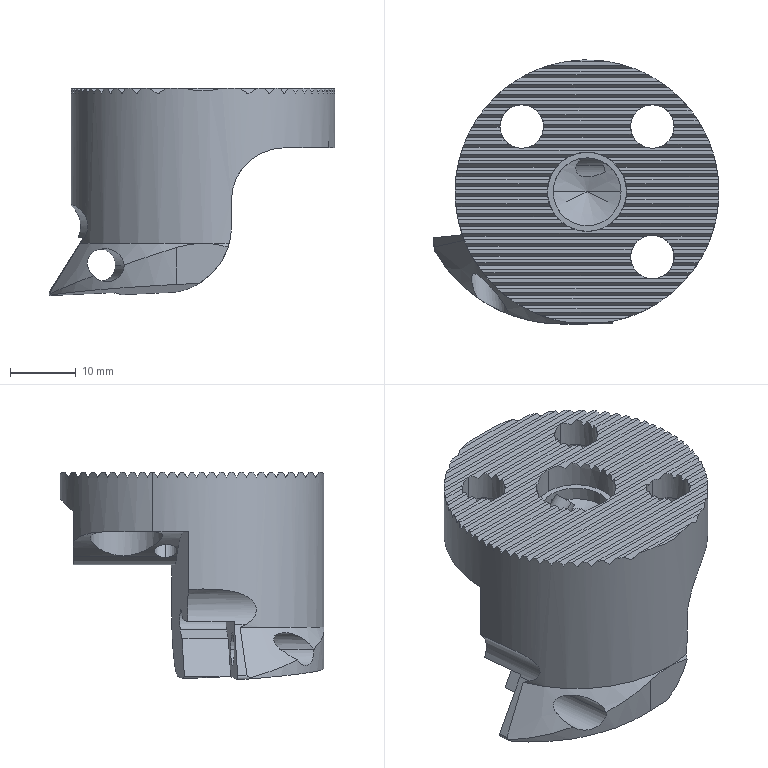Part | 1 solid | 196 faces | volume 18012 mm3 | plane 160 | cylinder 32 | cone 4 | commonest cylinder face diameters 6.6 x6 11 x6 3.4 x3 5 x2 8 x2 10.3 x2